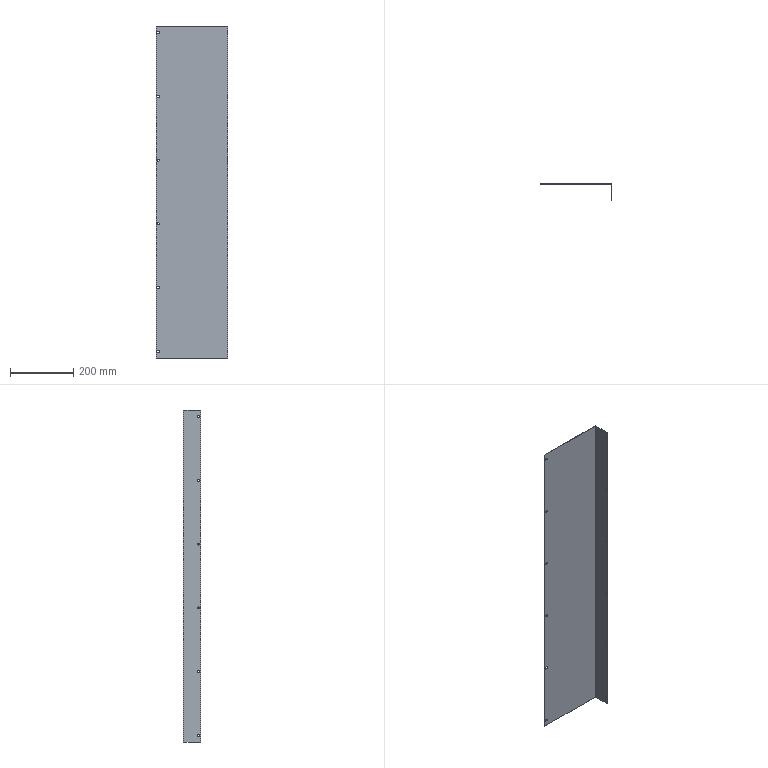Part | 1 solid | 74 faces | box 227.5 x 54 x 1050 mm | volume 293654 mm3 | cylinder 38 | plane 36 | commonest cylinder face diameters 6 x36 0.4 x1 2.4 x1